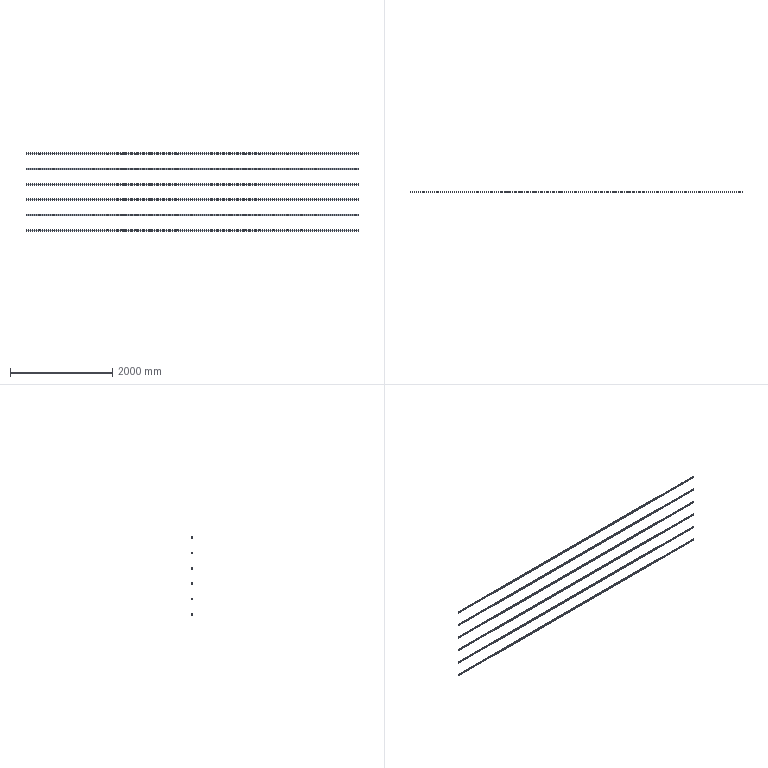Part | SolidWorks | features 3DProfileFeature 1, Cut 1, LPattern 1, WeldMemberFeat 1, WeldmentFeature 1 | 6 solids | 684 faces | box 6500 x 15 x 1530 mm | volume 5917812 mm3 | cylinder 624 | plane 60 | commonest cylinder face diameters 13 x576 4 x24 8 x24